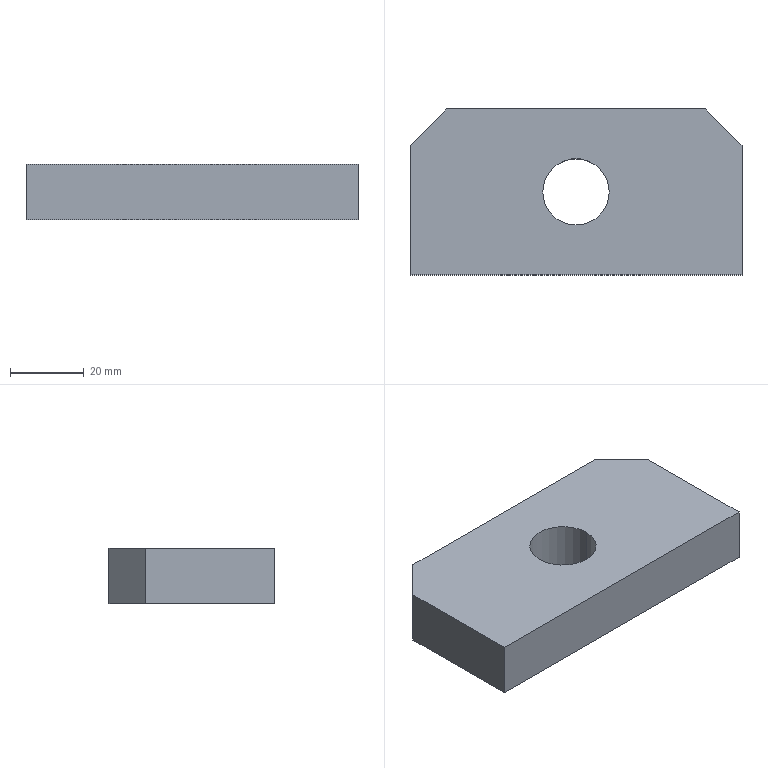Part | STEP file | 1 solid | 10 faces | box 90 x 45 x 15 mm | volume 55433 mm3 | plane 8 | cylinder 2 | commonest cylinder face diameters 18 x2
STEP:
#1=CARTESIAN_POINT('',(0.,0.,0.));
#2=DIRECTION('',(0.,0.,1.));
#3=DIRECTION('',(1.,0.,0.));
#4=AXIS2_PLACEMENT_3D('',#1,#2,#3);
#5=CARTESIAN_POINT('',(9.,0.,15.));
#6=VERTEX_POINT('',#5);
#7=CARTESIAN_POINT('',(-9.,0.,15.));
#8=VERTEX_POINT('',#7);
#9=CARTESIAN_POINT('',(0.,0.,15.));
#10=DIRECTION('',(0.,0.,-1.));
#11=DIRECTION('',(1.,0.,0.));
#12=AXIS2_PLACEMENT_3D('',#9,#10,#11);
#13=CIRCLE('',#12,9.);
#14=CARTESIAN_POINT('',(0.,0.,15.));
#15=DIRECTION('',(0.,0.,-1.));
#16=DIRECTION('',(0.,-1.,0.));
#17=AXIS2_PLACEMENT_3D('',#14,#15,#16);
#18=PLANE('',#17);
#19=CARTESIAN_POINT('',(0.,0.));
#20=DIRECTION('',(0.,-1.));
#21=AXIS2_PLACEMENT_2D('',#19,#20);
#22=CIRCLE('',#21,9.);
#23=(GEOMETRIC_REPRESENTATION_CONTEXT(2)PARAMETRIC_REPRESENTATION_CONTEXT()REPRESENTATION_CONTEXT('',''));
#24=DEFINITIONAL_REPRESENTATION('',(#22),#23);
#25=PCURVE('',#18,#24);
#26=CARTESIAN_POINT('',(0.,0.,15.));
#27=DIRECTION('',(0.,0.,1.));
#28=DIRECTION('',(1.,0.,0.));
#29=AXIS2_PLACEMENT_3D('',#26,#27,#28);
#30=CYLINDRICAL_SURFACE('',#29,9.);
#31=CARTESIAN_POINT('',(6.283,0.));
#32=DIRECTION('',(-1.,0.));
#33=VECTOR('',#32,1.);
#34=LINE('',#31,#33);
#35=(GEOMETRIC_REPRESENTATION_CONTEXT(2)PARAMETRIC_REPRESENTATION_CONTEXT()REPRESENTATION_CONTEXT('',''));
#36=DEFINITIONAL_REPRESENTATION('',(#34),#35);
#37=PCURVE('',#30,#36);
#38=SURFACE_CURVE('',#13,(#25,#37),.PCURVE_S1.);
#39=EDGE_CURVE('',#6,#8,#38,.T.);
#40=ORIENTED_EDGE('',*,*,#39,.T.);
#41=CARTESIAN_POINT('',(0.,0.,15.));
#42=DIRECTION('',(0.,0.,-1.));
#43=DIRECTION('',(1.,0.,0.));
#44=AXIS2_PLACEMENT_3D('',#41,#42,#43);
#45=CIRCLE('',#44,9.);
#46=CARTESIAN_POINT('',(0.,0.));
#47=DIRECTION('',(0.,-1.));
#48=AXIS2_PLACEMENT_2D('',#46,#47);
#49=CIRCLE('',#48,9.);
#50=(GEOMETRIC_REPRESENTATION_CONTEXT(2)PARAMETRIC_REPRESENTATION_CONTEXT()REPRESENTATION_CONTEXT('',''));
#51=DEFINITIONAL_REPRESENTATION('',(#49),#50);
#52=PCURVE('',#18,#51);
#53=CARTESIAN_POINT('',(0.,0.,15.));
#54=DIRECTION('',(0.,0.,1.));
#55=DIRECTION('',(1.,0.,0.));
#56=AXIS2_PLACEMENT_3D('',#53,#54,#55);
#57=CYLINDRICAL_SURFACE('',#56,9.);
#58=CARTESIAN_POINT('',(6.283,0.));
#59=DIRECTION('',(-1.,0.));
#60=VECTOR('',#59,1.);
#61=LINE('',#58,#60);
#62=(GEOMETRIC_REPRESENTATION_CONTEXT(2)PARAMETRIC_REPRESENTATION_CONTEXT()REPRESENTATION_CONTEXT('',''));
#63=DEFINITIONAL_REPRESENTATION('',(#61),#62);
#64=PCURVE('',#57,#63);
#65=SURFACE_CURVE('',#45,(#52,#64),.PCURVE_S1.);
#66=EDGE_CURVE('',#8,#6,#65,.T.);
#67=ORIENTED_EDGE('',*,*,#66,.T.);
#68=EDGE_LOOP('',(#40,#67));
#69=FACE_BOUND('',#68,.T.);
#70=CARTESIAN_POINT('',(35.,22.5,15.));
#71=VERTEX_POINT('',#70);
#72=CARTESIAN_POINT('',(-35.,22.5,15.));
#73=VERTEX_POINT('',#72);
#74=CARTESIAN_POINT('',(35.,22.5,15.));
#75=DIRECTION('',(-1.,0.,0.));
#76=VECTOR('',#75,1.);
#77=LINE('',#74,#76);
#78=CARTESIAN_POINT('',(-22.5,-35.));
#79=DIRECTION('',(0.,1.));
#80=VECTOR('',#79,1.);
#81=LINE('',#78,#80);
#82=(GEOMETRIC_REPRESENTATION_CONTEXT(2)PARAMETRIC_REPRESENTATION_CONTEXT()REPRESENTATION_CONTEXT('',''));
#83=DEFINITIONAL_REPRESENTATION('',(#81),#82);
#84=PCURVE('',#18,#83);
#85=CARTESIAN_POINT('',(35.,22.5,15.));
#86=DIRECTION('',(0.,-1.,0.));
#87=DIRECTION('',(0.,0.,-1.));
#88=AXIS2_PLACEMENT_3D('',#85,#86,#87);
#89=PLANE('',#88);
#90=CARTESIAN_POINT('',(0.,0.));
#91=DIRECTION('',(0.,-1.));
#92=VECTOR('',#91,1.);
#93=LINE('',#90,#92);
#94=(GEOMETRIC_REPRESENTATION_CONTEXT(2)PARAMETRIC_REPRESENTATION_CONTEXT()REPRESENTATION_CONTEXT('',''));
#95=DEFINITIONAL_REPRESENTATION('',(#93),#94);
#96=PCURVE('',#89,#95);
#97=SURFACE_CURVE('',#77,(#84,#96),.PCURVE_S1.);
#98=EDGE_CURVE('',#71,#73,#97,.T.);
#99=ORIENTED_EDGE('',*,*,#98,.T.);
#100=CARTESIAN_POINT('',(-45.,12.5,15.));
#101=VERTEX_POINT('',#100);
#102=CARTESIAN_POINT('',(-45.,12.5,15.));
#103=DIRECTION('',(0.7071,0.7071,0.));
#104=VECTOR('',#103,1.);
#105=LINE('',#102,#104);
#106=CARTESIAN_POINT('',(-12.5,45.));
#107=DIRECTION('',(-0.7071,-0.7071));
#108=VECTOR('',#107,1.);
#109=LINE('',#106,#108);
#110=(GEOMETRIC_REPRESENTATION_CONTEXT(2)PARAMETRIC_REPRESENTATION_CONTEXT()REPRESENTATION_CONTEXT('',''));
#111=DEFINITIONAL_REPRESENTATION('',(#109),#110);
#112=PCURVE('',#18,#111);
#113=CARTESIAN_POINT('',(-45.,12.5,15.));
#114=DIRECTION('',(-0.7071,0.7071,0.));
#115=DIRECTION('',(0.,0.,1.));
#116=AXIS2_PLACEMENT_3D('',#113,#114,#115);
#117=PLANE('',#116);
#118=CARTESIAN_POINT('',(0.,0.));
#119=DIRECTION('',(0.,1.));
#120=VECTOR('',#119,1.);
#121=LINE('',#118,#120);
#122=(GEOMETRIC_REPRESENTATION_CONTEXT(2)PARAMETRIC_REPRESENTATION_CONTEXT()REPRESENTATION_CONTEXT('',''));
#123=DEFINITIONAL_REPRESENTATION('',(#121),#122);
#124=PCURVE('',#117,#123);
#125=SURFACE_CURVE('',#105,(#112,#124),.PCURVE_S1.);
#126=EDGE_CURVE('',#101,#73,#125,.T.);
#127=ORIENTED_EDGE('',*,*,#126,.F.);
#128=CARTESIAN_POINT('',(-45.,-22.5,15.));
#129=VERTEX_POINT('',#128);
#130=CARTESIAN_POINT('',(-45.,-22.5,15.));
#131=DIRECTION('',(0.,1.,0.));
#132=VECTOR('',#131,1.);
#133=LINE('',#130,#132);
#134=CARTESIAN_POINT('',(22.5,45.));
#135=DIRECTION('',(-1.,0.));
#136=VECTOR('',#135,1.);
#137=LINE('',#134,#136);
#138=(GEOMETRIC_REPRESENTATION_CONTEXT(2)PARAMETRIC_REPRESENTATION_CONTEXT()REPRESENTATION_CONTEXT('',''));
#139=DEFINITIONAL_REPRESENTATION('',(#137),#138);
#140=PCURVE('',#18,#139);
#141=CARTESIAN_POINT('',(-45.,-22.5,15.));
#142=DIRECTION('',(-1.,0.,0.));
#143=DIRECTION('',(0.,0.,1.));
#144=AXIS2_PLACEMENT_3D('',#141,#142,#143);
#145=PLANE('',#144);
#146=CARTESIAN_POINT('',(0.,0.));
#147=DIRECTION('',(0.,1.));
#148=VECTOR('',#147,1.);
#149=LINE('',#146,#148);
#150=(GEOMETRIC_REPRESENTATION_CONTEXT(2)PARAMETRIC_REPRESENTATION_CONTEXT()REPRESENTATION_CONTEXT('',''));
#151=DEFINITIONAL_REPRESENTATION('',(#149),#150);
#152=PCURVE('',#145,#151);
#153=SURFACE_CURVE('',#133,(#140,#152),.PCURVE_S1.);
#154=EDGE_CURVE('',#129,#101,#153,.T.);
#155=ORIENTED_EDGE('',*,*,#154,.F.);
#156=CARTESIAN_POINT('',(45.,-22.5,15.));
#157=VERTEX_POINT('',#156);
#158=CARTESIAN_POINT('',(45.,-22.5,15.));
#159=DIRECTION('',(-1.,0.,0.));
#160=VECTOR('',#159,1.);
#161=LINE('',#158,#160);
#162=CARTESIAN_POINT('',(22.5,-45.));
#163=DIRECTION('',(0.,1.));
#164=VECTOR('',#163,1.);
#165=LINE('',#162,#164);
#166=(GEOMETRIC_REPRESENTATION_CONTEXT(2)PARAMETRIC_REPRESENTATION_CONTEXT()REPRESENTATION_CONTEXT('',''));
#167=DEFINITIONAL_REPRESENTATION('',(#165),#166);
#168=PCURVE('',#18,#167);
#169=CARTESIAN_POINT('',(45.,-22.5,15.));
#170=DIRECTION('',(0.,-1.,0.));
#171=DIRECTION('',(0.,0.,-1.));
#172=AXIS2_PLACEMENT_3D('',#169,#170,#171);
#173=PLANE('',#172);
#174=CARTESIAN_POINT('',(0.,0.));
#175=DIRECTION('',(0.,-1.));
#176=VECTOR('',#175,1.);
#177=LINE('',#174,#176);
#178=(GEOMETRIC_REPRESENTATION_CONTEXT(2)PARAMETRIC_REPRESENTATION_CONTEXT()REPRESENTATION_CONTEXT('',''));
#179=DEFINITIONAL_REPRESENTATION('',(#177),#178);
#180=PCURVE('',#173,#179);
#181=SURFACE_CURVE('',#161,(#168,#180),.PCURVE_S1.);
#182=EDGE_CURVE('',#157,#129,#181,.T.);
#183=ORIENTED_EDGE('',*,*,#182,.F.);
#184=CARTESIAN_POINT('',(45.,12.5,15.));
#185=VERTEX_POINT('',#184);
#186=CARTESIAN_POINT('',(45.,-22.5,15.));
#187=DIRECTION('',(0.,1.,0.));
#188=VECTOR('',#187,1.);
#189=LINE('',#186,#188);
#190=CARTESIAN_POINT('',(22.5,-45.));
#191=DIRECTION('',(-1.,0.));
#192=VECTOR('',#191,1.);
#193=LINE('',#190,#192);
#194=(GEOMETRIC_REPRESENTATION_CONTEXT(2)PARAMETRIC_REPRESENTATION_CONTEXT()REPRESENTATION_CONTEXT('',''));
#195=DEFINITIONAL_REPRESENTATION('',(#193),#194);
#196=PCURVE('',#18,#195);
#197=CARTESIAN_POINT('',(45.,-22.5,15.));
#198=DIRECTION('',(-1.,0.,0.));
#199=DIRECTION('',(0.,0.,1.));
#200=AXIS2_PLACEMENT_3D('',#197,#198,#199);
#201=PLANE('',#200);
#202=CARTESIAN_POINT('',(0.,0.));
#203=DIRECTION('',(0.,1.));
#204=VECTOR('',#203,1.);
#205=LINE('',#202,#204);
#206=(GEOMETRIC_REPRESENTATION_CONTEXT(2)PARAMETRIC_REPRESENTATION_CONTEXT()REPRESENTATION_CONTEXT('',''));
#207=DEFINITIONAL_REPRESENTATION('',(#205),#206);
#208=PCURVE('',#201,#207);
#209=SURFACE_CURVE('',#189,(#196,#208),.PCURVE_S1.);
#210=EDGE_CURVE('',#157,#185,#209,.T.);
#211=ORIENTED_EDGE('',*,*,#210,.T.);
#212=CARTESIAN_POINT('',(45.,12.5,15.));
#213=DIRECTION('',(-0.7071,0.7071,0.));
#214=VECTOR('',#213,1.);
#215=LINE('',#212,#214);
#216=CARTESIAN_POINT('',(-12.5,-45.));
#217=DIRECTION('',(-0.7071,0.7071));
#218=VECTOR('',#217,1.);
#219=LINE('',#216,#218);
#220=(GEOMETRIC_REPRESENTATION_CONTEXT(2)PARAMETRIC_REPRESENTATION_CONTEXT()REPRESENTATION_CONTEXT('',''));
#221=DEFINITIONAL_REPRESENTATION('',(#219),#220);
#222=PCURVE('',#18,#221);
#223=CARTESIAN_POINT('',(45.,12.5,15.));
#224=DIRECTION('',(-0.7071,-0.7071,0.));
#225=DIRECTION('',(-0.7071,0.7071,0.));
#226=AXIS2_PLACEMENT_3D('',#223,#224,#225);
#227=PLANE('',#226);
#228=CARTESIAN_POINT('',(0.,0.));
#229=DIRECTION('',(1.,0.));
#230=VECTOR('',#229,1.);
#231=LINE('',#228,#230);
#232=(GEOMETRIC_REPRESENTATION_CONTEXT(2)PARAMETRIC_REPRESENTATION_CONTEXT()REPRESENTATION_CONTEXT('',''));
#233=DEFINITIONAL_REPRESENTATION('',(#231),#232);
#234=PCURVE('',#227,#233);
#235=SURFACE_CURVE('',#215,(#222,#234),.PCURVE_S1.);
#236=EDGE_CURVE('',#185,#71,#235,.T.);
#237=ORIENTED_EDGE('',*,*,#236,.T.);
#238=EDGE_LOOP('',(#99,#127,#155,#183,#211,#237));
#239=FACE_BOUND('',#238,.T.);
#240=ADVANCED_FACE('',(#69,#239),#18,.F.);
#241=ORIENTED_EDGE('',*,*,#66,.T.);
#242=CARTESIAN_POINT('',(9.,0.,0.));
#243=VERTEX_POINT('',#242);
#244=CARTESIAN_POINT('',(9.,0.,15.));
#245=DIRECTION('',(0.,0.,1.));
#246=VECTOR('',#245,1.);
#247=LINE('',#244,#246);
#248=CARTESIAN_POINT('',(0.,0.));
#249=DIRECTION('',(0.,1.));
#250=VECTOR('',#249,1.);
#251=LINE('',#248,#250);
#252=(GEOMETRIC_REPRESENTATION_CONTEXT(2)PARAMETRIC_REPRESENTATION_CONTEXT()REPRESENTATION_CONTEXT('',''));
#253=DEFINITIONAL_REPRESENTATION('',(#251),#252);
#254=PCURVE('',#57,#253);
#255=CARTESIAN_POINT('',(6.283,0.));
#256=DIRECTION('',(0.,1.));
#257=VECTOR('',#256,1.);
#258=LINE('',#255,#257);
#259=(GEOMETRIC_REPRESENTATION_CONTEXT(2)PARAMETRIC_REPRESENTATION_CONTEXT()REPRESENTATION_CONTEXT('',''));
#260=DEFINITIONAL_REPRESENTATION('',(#258),#259);
#261=PCURVE('',#30,#260);
#262=SURFACE_CURVE('',#247,(#254,#261),.PCURVE_S1.);
#263=EDGE_CURVE('',#243,#6,#262,.T.);
#264=ORIENTED_EDGE('',*,*,#263,.F.);
#265=CARTESIAN_POINT('',(-9.,0.,0.));
#266=VERTEX_POINT('',#265);
#267=CARTESIAN_POINT('',(0.,0.,0.));
#268=DIRECTION('',(0.,0.,1.));
#269=DIRECTION('',(1.,0.,0.));
#270=AXIS2_PLACEMENT_3D('',#267,#268,#269);
#271=CIRCLE('',#270,9.);
#272=CARTESIAN_POINT('',(0.,-15.));
#273=DIRECTION('',(1.,0.));
#274=VECTOR('',#273,1.);
#275=LINE('',#272,#274);
#276=(GEOMETRIC_REPRESENTATION_CONTEXT(2)PARAMETRIC_REPRESENTATION_CONTEXT()REPRESENTATION_CONTEXT('',''));
#277=DEFINITIONAL_REPRESENTATION('',(#275),#276);
#278=PCURVE('',#57,#277);
#279=CARTESIAN_POINT('',(0.,0.,0.));
#280=DIRECTION('',(0.,0.,-1.));
#281=DIRECTION('',(0.,-1.,0.));
#282=AXIS2_PLACEMENT_3D('',#279,#280,#281);
#283=PLANE('',#282);
#284=CARTESIAN_POINT('',(0.,-9.));
#285=CARTESIAN_POINT('',(-15.588,-9.));
#286=CARTESIAN_POINT('',(-7.794,4.5));
#287=CARTESIAN_POINT('',(0.,18.));
#288=CARTESIAN_POINT('',(7.794,4.5));
#289=CARTESIAN_POINT('',(15.588,-9.));
#290=CARTESIAN_POINT('',(0.,-9.));
#291=(BOUNDED_CURVE()B_SPLINE_CURVE(2,(#284,#285,#286,#287,#288,#289,#290),.UNSPECIFIED.,.T.,.F.)B_SPLINE_CURVE_WITH_KNOTS((1,2,2,2,2,1),(-2.094,0.,2.094,4.189,6.283,8.378),.UNSPECIFIED.)CURVE()GEOMETRIC_REPRESENTATION_ITEM()RATIONAL_B_SPLINE_CURVE((1.,0.5,1.,0.5,1.,0.5,1.))REPRESENTATION_ITEM(''));
#292=(GEOMETRIC_REPRESENTATION_CONTEXT(2)PARAMETRIC_REPRESENTATION_CONTEXT()REPRESENTATION_CONTEXT('',''));
#293=DEFINITIONAL_REPRESENTATION('',(#291),#292);
#294=PCURVE('',#283,#293);
#295=SURFACE_CURVE('',#271,(#278,#294),.PCURVE_S1.);
#296=EDGE_CURVE('',#243,#266,#295,.T.);
#297=ORIENTED_EDGE('',*,*,#296,.T.);
#298=CARTESIAN_POINT('',(-9.,0.,15.));
#299=DIRECTION('',(0.,0.,1.));
#300=VECTOR('',#299,1.);
#301=LINE('',#298,#300);
#302=CARTESIAN_POINT('',(3.142,0.));
#303=DIRECTION('',(0.,1.));
#304=VECTOR('',#303,1.);
#305=LINE('',#302,#304);
#306=(GEOMETRIC_REPRESENTATION_CONTEXT(2)PARAMETRIC_REPRESENTATION_CONTEXT()REPRESENTATION_CONTEXT('',''));
#307=DEFINITIONAL_REPRESENTATION('',(#305),#306);
#308=PCURVE('',#57,#307);
#309=CARTESIAN_POINT('',(3.142,0.));
#310=DIRECTION('',(0.,1.));
#311=VECTOR('',#310,1.);
#312=LINE('',#309,#311);
#313=(GEOMETRIC_REPRESENTATION_CONTEXT(2)PARAMETRIC_REPRESENTATION_CONTEXT()REPRESENTATION_CONTEXT('',''));
#314=DEFINITIONAL_REPRESENTATION('',(#312),#313);
#315=PCURVE('',#30,#314);
#316=SURFACE_CURVE('',#301,(#308,#315),.PCURVE_S1.);
#317=EDGE_CURVE('',#266,#8,#316,.T.);
#318=ORIENTED_EDGE('',*,*,#317,.T.);
#319=EDGE_LOOP('',(#241,#264,#297,#318));
#320=FACE_BOUND('',#319,.F.);
#321=ADVANCED_FACE('',(#320),#57,.F.);
#322=CARTESIAN_POINT('',(35.,22.5,0.));
#323=VERTEX_POINT('',#322);
#324=CARTESIAN_POINT('',(35.,22.5,15.));
#325=DIRECTION('',(0.,0.,1.));
#326=VECTOR('',#325,1.);
#327=LINE('',#324,#326);
#328=CARTESIAN_POINT('',(14.142,0.));
#329=DIRECTION('',(0.,-1.));
#330=VECTOR('',#329,1.);
#331=LINE('',#328,#330);
#332=(GEOMETRIC_REPRESENTATION_CONTEXT(2)PARAMETRIC_REPRESENTATION_CONTEXT()REPRESENTATION_CONTEXT('',''));
#333=DEFINITIONAL_REPRESENTATION('',(#331),#332);
#334=PCURVE('',#227,#333);
#335=CARTESIAN_POINT('',(0.,0.));
#336=DIRECTION('',(-1.,0.));
#337=VECTOR('',#336,1.);
#338=LINE('',#335,#337);
#339=(GEOMETRIC_REPRESENTATION_CONTEXT(2)PARAMETRIC_REPRESENTATION_CONTEXT()REPRESENTATION_CONTEXT('',''));
#340=DEFINITIONAL_REPRESENTATION('',(#338),#339);
#341=PCURVE('',#89,#340);
#342=SURFACE_CURVE('',#327,(#334,#341),.PCURVE_S1.);
#343=EDGE_CURVE('',#323,#71,#342,.T.);
#344=ORIENTED_EDGE('',*,*,#343,.T.);
#345=ORIENTED_EDGE('',*,*,#236,.F.);
#346=CARTESIAN_POINT('',(45.,12.5,0.));
#347=VERTEX_POINT('',#346);
#348=CARTESIAN_POINT('',(45.,12.5,15.));
#349=DIRECTION('',(0.,0.,-1.));
#350=VECTOR('',#349,1.);
#351=LINE('',#348,#350);
#352=CARTESIAN_POINT('',(0.,0.));
#353=DIRECTION('',(0.,1.));
#354=VECTOR('',#353,1.);
#355=LINE('',#352,#354);
#356=(GEOMETRIC_REPRESENTATION_CONTEXT(2)PARAMETRIC_REPRESENTATION_CONTEXT()REPRESENTATION_CONTEXT('',''));
#357=DEFINITIONAL_REPRESENTATION('',(#355),#356);
#358=PCURVE('',#227,#357);
#359=CARTESIAN_POINT('',(0.,35.));
#360=DIRECTION('',(-1.,0.));
#361=VECTOR('',#360,1.);
#362=LINE('',#359,#361);
#363=(GEOMETRIC_REPRESENTATION_CONTEXT(2)PARAMETRIC_REPRESENTATION_CONTEXT()REPRESENTATION_CONTEXT('',''));
#364=DEFINITIONAL_REPRESENTATION('',(#362),#363);
#365=PCURVE('',#201,#364);
#366=SURFACE_CURVE('',#351,(#358,#365),.PCURVE_S1.);
#367=EDGE_CURVE('',#185,#347,#366,.T.);
#368=ORIENTED_EDGE('',*,*,#367,.T.);
#369=CARTESIAN_POINT('',(35.,22.5,0.));
#370=DIRECTION('',(0.7071,-0.7071,0.));
#371=VECTOR('',#370,1.);
#372=LINE('',#369,#371);
#373=CARTESIAN_POINT('',(14.142,15.));
#374=DIRECTION('',(-1.,0.));
#375=VECTOR('',#374,1.);
#376=LINE('',#373,#375);
#377=(GEOMETRIC_REPRESENTATION_CONTEXT(2)PARAMETRIC_REPRESENTATION_CONTEXT()REPRESENTATION_CONTEXT('',''));
#378=DEFINITIONAL_REPRESENTATION('',(#376),#377);
#379=PCURVE('',#227,#378);
#380=CARTESIAN_POINT('',(-22.5,-35.));
#381=DIRECTION('',(0.7071,-0.7071));
#382=VECTOR('',#381,1.);
#383=LINE('',#380,#382);
#384=(GEOMETRIC_REPRESENTATION_CONTEXT(2)PARAMETRIC_REPRESENTATION_CONTEXT()REPRESENTATION_CONTEXT('',''));
#385=DEFINITIONAL_REPRESENTATION('',(#383),#384);
#386=PCURVE('',#283,#385);
#387=SURFACE_CURVE('',#372,(#379,#386),.PCURVE_S1.);
#388=EDGE_CURVE('',#323,#347,#387,.T.);
#389=ORIENTED_EDGE('',*,*,#388,.F.);
#390=EDGE_LOOP('',(#344,#345,#368,#389));
#391=FACE_BOUND('',#390,.T.);
#392=ADVANCED_FACE('',(#391),#227,.F.);
#393=ORIENTED_EDGE('',*,*,#367,.F.);
#394=ORIENTED_EDGE('',*,*,#210,.F.);
#395=CARTESIAN_POINT('',(45.,-22.5,0.));
#396=VERTEX_POINT('',#395);
#397=CARTESIAN_POINT('',(45.,-22.5,15.));
#398=DIRECTION('',(0.,0.,1.));
#399=VECTOR('',#398,1.);
#400=LINE('',#397,#399);
#401=CARTESIAN_POINT('',(0.,0.));
#402=DIRECTION('',(1.,0.));
#403=VECTOR('',#402,1.);
#404=LINE('',#401,#403);
#405=(GEOMETRIC_REPRESENTATION_CONTEXT(2)PARAMETRIC_REPRESENTATION_CONTEXT()REPRESENTATION_CONTEXT('',''));
#406=DEFINITIONAL_REPRESENTATION('',(#404),#405);
#407=PCURVE('',#201,#406);
#408=CARTESIAN_POINT('',(0.,0.));
#409=DIRECTION('',(-1.,0.));
#410=VECTOR('',#409,1.);
#411=LINE('',#408,#410);
#412=(GEOMETRIC_REPRESENTATION_CONTEXT(2)PARAMETRIC_REPRESENTATION_CONTEXT()REPRESENTATION_CONTEXT('',''));
#413=DEFINITIONAL_REPRESENTATION('',(#411),#412);
#414=PCURVE('',#173,#413);
#415=SURFACE_CURVE('',#400,(#407,#414),.PCURVE_S1.);
#416=EDGE_CURVE('',#396,#157,#415,.T.);
#417=ORIENTED_EDGE('',*,*,#416,.F.);
#418=CARTESIAN_POINT('',(45.,0.,0.));
#419=DIRECTION('',(0.,-1.,0.));
#420=VECTOR('',#419,1.);
#421=LINE('',#418,#420);
#422=CARTESIAN_POINT('',(-15.,22.5));
#423=DIRECTION('',(0.,-1.));
#424=VECTOR('',#423,1.);
#425=LINE('',#422,#424);
#426=(GEOMETRIC_REPRESENTATION_CONTEXT(2)PARAMETRIC_REPRESENTATION_CONTEXT()REPRESENTATION_CONTEXT('',''));
#427=DEFINITIONAL_REPRESENTATION('',(#425),#426);
#428=PCURVE('',#201,#427);
#429=CARTESIAN_POINT('',(0.,-45.));
#430=DIRECTION('',(1.,0.));
#431=VECTOR('',#430,1.);
#432=LINE('',#429,#431);
#433=(GEOMETRIC_REPRESENTATION_CONTEXT(2)PARAMETRIC_REPRESENTATION_CONTEXT()REPRESENTATION_CONTEXT('',''));
#434=DEFINITIONAL_REPRESENTATION('',(#432),#433);
#435=PCURVE('',#283,#434);
#436=SURFACE_CURVE('',#421,(#428,#435),.PCURVE_S1.);
#437=EDGE_CURVE('',#347,#396,#436,.T.);
#438=ORIENTED_EDGE('',*,*,#437,.F.);
#439=EDGE_LOOP('',(#393,#394,#417,#438));
#440=FACE_BOUND('',#439,.T.);
#441=ADVANCED_FACE('',(#440),#201,.F.);
#442=ORIENTED_EDGE('',*,*,#182,.T.);
#443=CARTESIAN_POINT('',(-45.,-22.5,0.));
#444=VERTEX_POINT('',#443);
#445=CARTESIAN_POINT('',(-45.,-22.5,15.));
#446=DIRECTION('',(0.,0.,1.));
#447=VECTOR('',#446,1.);
#448=LINE('',#445,#447);
#449=CARTESIAN_POINT('',(0.,-90.));
#450=DIRECTION('',(-1.,0.));
#451=VECTOR('',#450,1.);
#452=LINE('',#449,#451);
#453=(GEOMETRIC_REPRESENTATION_CONTEXT(2)PARAMETRIC_REPRESENTATION_CONTEXT()REPRESENTATION_CONTEXT('',''));
#454=DEFINITIONAL_REPRESENTATION('',(#452),#453);
#455=PCURVE('',#173,#454);
#456=CARTESIAN_POINT('',(0.,0.));
#457=DIRECTION('',(1.,0.));
#458=VECTOR('',#457,1.);
#459=LINE('',#456,#458);
#460=(GEOMETRIC_REPRESENTATION_CONTEXT(2)PARAMETRIC_REPRESENTATION_CONTEXT()REPRESENTATION_CONTEXT('',''));
#461=DEFINITIONAL_REPRESENTATION('',(#459),#460);
#462=PCURVE('',#145,#461);
#463=SURFACE_CURVE('',#448,(#455,#462),.PCURVE_S1.);
#464=EDGE_CURVE('',#444,#129,#463,.T.);
#465=ORIENTED_EDGE('',*,*,#464,.F.);
#466=CARTESIAN_POINT('',(0.,-22.5,0.));
#467=DIRECTION('',(-1.,0.,0.));
#468=VECTOR('',#467,1.);
#469=LINE('',#466,#468);
#470=CARTESIAN_POINT('',(15.,-45.));
#471=DIRECTION('',(0.,-1.));
#472=VECTOR('',#471,1.);
#473=LINE('',#470,#472);
#474=(GEOMETRIC_REPRESENTATION_CONTEXT(2)PARAMETRIC_REPRESENTATION_CONTEXT()REPRESENTATION_CONTEXT('',''));
#475=DEFINITIONAL_REPRESENTATION('',(#473),#474);
#476=PCURVE('',#173,#475);
#477=CARTESIAN_POINT('',(22.5,0.));
#478=DIRECTION('',(0.,1.));
#479=VECTOR('',#478,1.);
#480=LINE('',#477,#479);
#481=(GEOMETRIC_REPRESENTATION_CONTEXT(2)PARAMETRIC_REPRESENTATION_CONTEXT()REPRESENTATION_CONTEXT('',''));
#482=DEFINITIONAL_REPRESENTATION('',(#480),#481);
#483=PCURVE('',#283,#482);
#484=SURFACE_CURVE('',#469,(#476,#483),.PCURVE_S1.);
#485=EDGE_CURVE('',#396,#444,#484,.T.);
#486=ORIENTED_EDGE('',*,*,#485,.F.);
#487=ORIENTED_EDGE('',*,*,#416,.T.);
#488=EDGE_LOOP('',(#442,#465,#486,#487));
#489=FACE_BOUND('',#488,.T.);
#490=ADVANCED_FACE('',(#489),#173,.T.);
#491=ORIENTED_EDGE('',*,*,#154,.T.);
#492=CARTESIAN_POINT('',(-45.,12.5,0.));
#493=VERTEX_POINT('',#492);
#494=CARTESIAN_POINT('',(-45.,12.5,15.));
#495=DIRECTION('',(0.,0.,1.));
#496=VECTOR('',#495,1.);
#497=LINE('',#494,#496);
#498=CARTESIAN_POINT('',(0.,35.));
#499=DIRECTION('',(1.,0.));
#500=VECTOR('',#499,1.);
#501=LINE('',#498,#500);
#502=(GEOMETRIC_REPRESENTATION_CONTEXT(2)PARAMETRIC_REPRESENTATION_CONTEXT()REPRESENTATION_CONTEXT('',''));
#503=DEFINITIONAL_REPRESENTATION('',(#501),#502);
#504=PCURVE('',#145,#503);
#505=CARTESIAN_POINT('',(0.,0.));
#506=DIRECTION('',(1.,0.));
#507=VECTOR('',#506,1.);
#508=LINE('',#505,#507);
#509=(GEOMETRIC_REPRESENTATION_CONTEXT(2)PARAMETRIC_REPRESENTATION_CONTEXT()REPRESENTATION_CONTEXT('',''));
#510=DEFINITIONAL_REPRESENTATION('',(#508),#509);
#511=PCURVE('',#117,#510);
#512=SURFACE_CURVE('',#497,(#504,#511),.PCURVE_S1.);
#513=EDGE_CURVE('',#493,#101,#512,.T.);
#514=ORIENTED_EDGE('',*,*,#513,.F.);
#515=CARTESIAN_POINT('',(-45.,0.,0.));
#516=DIRECTION('',(0.,1.,0.));
#517=VECTOR('',#516,1.);
#518=LINE('',#515,#517);
#519=CARTESIAN_POINT('',(-15.,22.5));
#520=DIRECTION('',(0.,1.));
#521=VECTOR('',#520,1.);
#522=LINE('',#519,#521);
#523=(GEOMETRIC_REPRESENTATION_CONTEXT(2)PARAMETRIC_REPRESENTATION_CONTEXT()REPRESENTATION_CONTEXT('',''));
#524=DEFINITIONAL_REPRESENTATION('',(#522),#523);
#525=PCURVE('',#145,#524);
#526=CARTESIAN_POINT('',(0.,45.));
#527=DIRECTION('',(-1.,0.));
#528=VECTOR('',#527,1.);
#529=LINE('',#526,#528);
#530=(GEOMETRIC_REPRESENTATION_CONTEXT(2)PARAMETRIC_REPRESENTATION_CONTEXT()REPRESENTATION_CONTEXT('',''));
#531=DEFINITIONAL_REPRESENTATION('',(#529),#530);
#532=PCURVE('',#283,#531);
#533=SURFACE_CURVE('',#518,(#525,#532),.PCURVE_S1.);
#534=EDGE_CURVE('',#444,#493,#533,.T.);
#535=ORIENTED_EDGE('',*,*,#534,.F.);
#536=ORIENTED_EDGE('',*,*,#464,.T.);
#537=EDGE_LOOP('',(#491,#514,#535,#536));
#538=FACE_BOUND('',#537,.T.);
#539=ADVANCED_FACE('',(#538),#145,.T.);
#540=ORIENTED_EDGE('',*,*,#126,.T.);
#541=CARTESIAN_POINT('',(-35.,22.5,0.));
#542=VERTEX_POINT('',#541);
#543=CARTESIAN_POINT('',(-35.,22.5,15.));
#544=DIRECTION('',(0.,0.,-1.));
#545=VECTOR('',#544,1.);
#546=LINE('',#543,#545);
#547=CARTESIAN_POINT('',(0.,14.142));
#548=DIRECTION('',(-1.,0.));
#549=VECTOR('',#548,1.);
#550=LINE('',#547,#549);
#551=(GEOMETRIC_REPRESENTATION_CONTEXT(2)PARAMETRIC_REPRESENTATION_CONTEXT()REPRESENTATION_CONTEXT('',''));
#552=DEFINITIONAL_REPRESENTATION('',(#550),#551);
#553=PCURVE('',#117,#552);
#554=CARTESIAN_POINT('',(0.,-70.));
#555=DIRECTION('',(1.,0.));
#556=VECTOR('',#555,1.);
#557=LINE('',#554,#556);
#558=(GEOMETRIC_REPRESENTATION_CONTEXT(2)PARAMETRIC_REPRESENTATION_CONTEXT()REPRESENTATION_CONTEXT('',''));
#559=DEFINITIONAL_REPRESENTATION('',(#557),#558);
#560=PCURVE('',#89,#559);
#561=SURFACE_CURVE('',#546,(#553,#560),.PCURVE_S1.);
#562=EDGE_CURVE('',#73,#542,#561,.T.);
#563=ORIENTED_EDGE('',*,*,#562,.T.);
#564=CARTESIAN_POINT('',(-45.,12.5,0.));
#565=DIRECTION('',(0.7071,0.7071,0.));
#566=VECTOR('',#565,1.);
#567=LINE('',#564,#566);
#568=CARTESIAN_POINT('',(-15.,0.));
#569=DIRECTION('',(0.,1.));
#570=VECTOR('',#569,1.);
#571=LINE('',#568,#570);
#572=(GEOMETRIC_REPRESENTATION_CONTEXT(2)PARAMETRIC_REPRESENTATION_CONTEXT()REPRESENTATION_CONTEXT('',''));
#573=DEFINITIONAL_REPRESENTATION('',(#571),#572);
#574=PCURVE('',#117,#573);
#575=CARTESIAN_POINT('',(-12.5,45.));
#576=DIRECTION('',(-0.7071,-0.7071));
#577=VECTOR('',#576,1.);
#578=LINE('',#575,#577);
#579=(GEOMETRIC_REPRESENTATION_CONTEXT(2)PARAMETRIC_REPRESENTATION_CONTEXT()REPRESENTATION_CONTEXT('',''));
#580=DEFINITIONAL_REPRESENTATION('',(#578),#579);
#581=PCURVE('',#283,#580);
#582=SURFACE_CURVE('',#567,(#574,#581),.PCURVE_S1.);
#583=EDGE_CURVE('',#493,#542,#582,.T.);
#584=ORIENTED_EDGE('',*,*,#583,.F.);
#585=ORIENTED_EDGE('',*,*,#513,.T.);
#586=EDGE_LOOP('',(#540,#563,#584,#585));
#587=FACE_BOUND('',#586,.T.);
#588=ADVANCED_FACE('',(#587),#117,.T.);
#589=ORIENTED_EDGE('',*,*,#562,.F.);
#590=ORIENTED_EDGE('',*,*,#98,.F.);
#591=ORIENTED_EDGE('',*,*,#343,.F.);
#592=CARTESIAN_POINT('',(0.,22.5,0.));
#593=DIRECTION('',(1.,0.,0.));
#594=VECTOR('',#593,1.);
#595=LINE('',#592,#594);
#596=CARTESIAN_POINT('',(15.,-35.));
#597=DIRECTION('',(0.,1.));
#598=VECTOR('',#597,1.);
#599=LINE('',#596,#598);
#600=(GEOMETRIC_REPRESENTATION_CONTEXT(2)PARAMETRIC_REPRESENTATION_CONTEXT()REPRESENTATION_CONTEXT('',''));
#601=DEFINITIONAL_REPRESENTATION('',(#599),#600);
#602=PCURVE('',#89,#601);
#603=CARTESIAN_POINT('',(-22.5,0.));
#604=DIRECTION('',(0.,-1.));
#605=VECTOR('',#604,1.);
#606=LINE('',#603,#605);
#607=(GEOMETRIC_REPRESENTATION_CONTEXT(2)PARAMETRIC_REPRESENTATION_CONTEXT()REPRESENTATION_CONTEXT('',''));
#608=DEFINITIONAL_REPRESENTATION('',(#606),#607);
#609=PCURVE('',#283,#608);
#610=SURFACE_CURVE('',#595,(#602,#609),.PCURVE_S1.);
#611=EDGE_CURVE('',#542,#323,#610,.T.);
#612=ORIENTED_EDGE('',*,*,#611,.F.);
#613=EDGE_LOOP('',(#589,#590,#591,#612));
#614=FACE_BOUND('',#613,.T.);
#615=ADVANCED_FACE('',(#614),#89,.F.);
#616=ORIENTED_EDGE('',*,*,#296,.T.);
#617=CARTESIAN_POINT('',(0.,0.,0.));
#618=DIRECTION('',(0.,0.,1.));
#619=DIRECTION('',(1.,0.,0.));
#620=AXIS2_PLACEMENT_3D('',#617,#618,#619);
#621=CIRCLE('',#620,9.);
#622=CARTESIAN_POINT('',(0.,-9.));
#623=CARTESIAN_POINT('',(-15.588,-9.));
#624=CARTESIAN_POINT('',(-7.794,4.5));
#625=CARTESIAN_POINT('',(0.,18.));
#626=CARTESIAN_POINT('',(7.794,4.5));
#627=CARTESIAN_POINT('',(15.588,-9.));
#628=CARTESIAN_POINT('',(0.,-9.));
#629=(BOUNDED_CURVE()B_SPLINE_CURVE(2,(#622,#623,#624,#625,#626,#627,#628),.UNSPECIFIED.,.T.,.F.)B_SPLINE_CURVE_WITH_KNOTS((1,2,2,2,2,1),(-2.094,0.,2.094,4.189,6.283,8.378),.UNSPECIFIED.)CURVE()GEOMETRIC_REPRESENTATION_ITEM()RATIONAL_B_SPLINE_CURVE((1.,0.5,1.,0.5,1.,0.5,1.))REPRESENTATION_ITEM(''));
#630=(GEOMETRIC_REPRESENTATION_CONTEXT(2)PARAMETRIC_REPRESENTATION_CONTEXT()REPRESENTATION_CONTEXT('',''));
#631=DEFINITIONAL_REPRESENTATION('',(#629),#630);
#632=PCURVE('',#283,#631);
#633=CARTESIAN_POINT('',(0.,-15.));
#634=DIRECTION('',(1.,0.));
#635=VECTOR('',#634,1.);
#636=LINE('',#633,#635);
#637=(GEOMETRIC_REPRESENTATION_CONTEXT(2)PARAMETRIC_REPRESENTATION_CONTEXT()REPRESENTATION_CONTEXT('',''));
#638=DEFINITIONAL_REPRESENTATION('',(#636),#637);
#639=PCURVE('',#30,#638);
#640=SURFACE_CURVE('',#621,(#632,#639),.PCURVE_S1.);
#641=EDGE_CURVE('',#266,#243,#640,.T.);
#642=ORIENTED_EDGE('',*,*,#641,.T.);
#643=EDGE_LOOP('',(#616,#642));
#644=FACE_BOUND('',#643,.T.);
#645=ORIENTED_EDGE('',*,*,#583,.T.);
#646=ORIENTED_EDGE('',*,*,#611,.T.);
#647=ORIENTED_EDGE('',*,*,#388,.T.);
#648=ORIENTED_EDGE('',*,*,#437,.T.);
#649=ORIENTED_EDGE('',*,*,#485,.T.);
#650=ORIENTED_EDGE('',*,*,#534,.T.);
#651=EDGE_LOOP('',(#645,#646,#647,#648,#649,#650));
#652=FACE_BOUND('',#651,.T.);
#653=ADVANCED_FACE('',(#644,#652),#283,.T.);
#654=ORIENTED_EDGE('',*,*,#263,.T.);
#655=ORIENTED_EDGE('',*,*,#39,.T.);
#656=ORIENTED_EDGE('',*,*,#317,.F.);
#657=ORIENTED_EDGE('',*,*,#641,.T.);
#658=EDGE_LOOP('',(#654,#655,#656,#657));
#659=FACE_BOUND('',#658,.F.);
#660=ADVANCED_FACE('',(#659),#30,.F.);
#661=CLOSED_SHELL('',(#240,#321,#392,#441,#490,#539,#588,#615,#653,#660));
#662=MANIFOLD_SOLID_BREP('',#661);
#663=(LENGTH_UNIT()NAMED_UNIT(*)SI_UNIT(.MILLI.,.METRE.));
#664=UNCERTAINTY_MEASURE_WITH_UNIT(LENGTH_MEASURE(0.0000001),#663,'','');
#665=(NAMED_UNIT(*)PLANE_ANGLE_UNIT()SI_UNIT($,.RADIAN.));
#666=(NAMED_UNIT(*)SI_UNIT($,.STERADIAN.)SOLID_ANGLE_UNIT());
#667=(GEOMETRIC_REPRESENTATION_CONTEXT(3)GLOBAL_UNCERTAINTY_ASSIGNED_CONTEXT((#664))GLOBAL_UNIT_ASSIGNED_CONTEXT((#663,#665,#666))REPRESENTATION_CONTEXT('',''));
#668=ADVANCED_BREP_SHAPE_REPRESENTATION('',(#4,#662),#667);